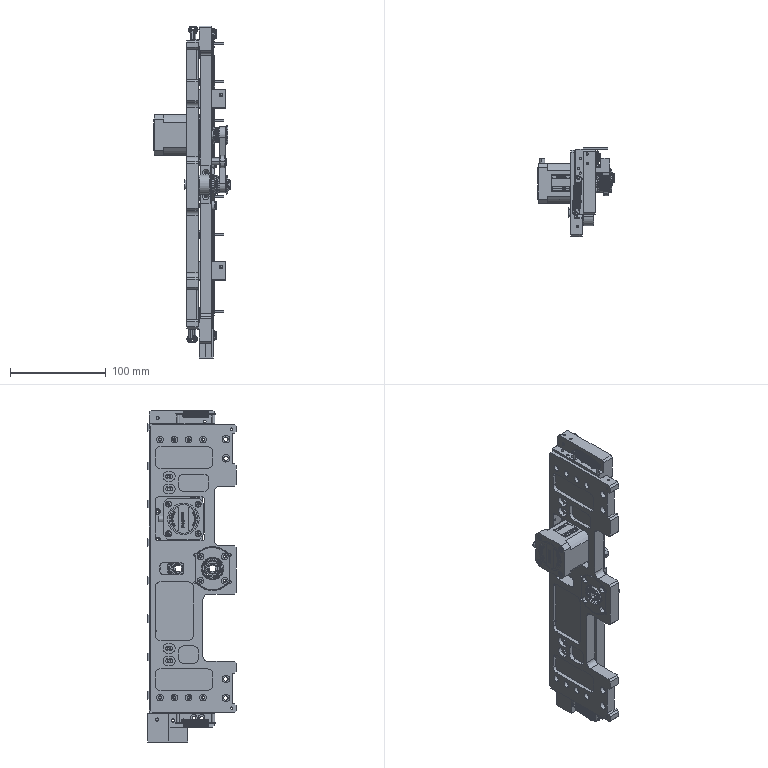Part | NX | features BREP 33 | 61 solids | 5049 faces | volume 466877 mm3 | plane 2453 | cylinder 1666 | spline 421 | cone 209 | sphere 180 | torus 120 | commonest cylinder face diameters 0.46 x382 4 x144 2.5 x112 3.4 x92 6 x88 10 x87